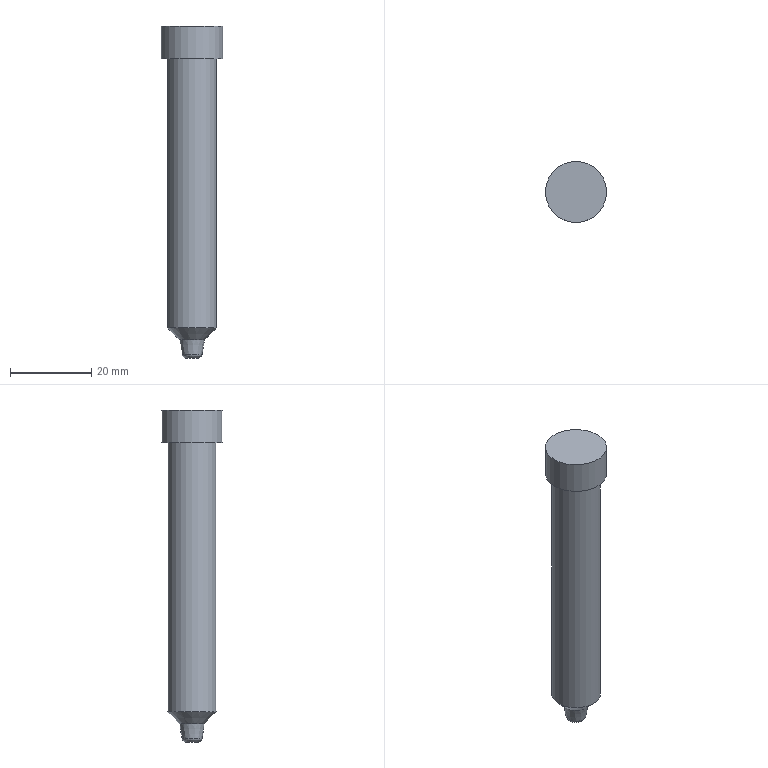Part | NX | features solid 2 | 1 solid | 8 faces | box 15 x 15 x 81.5 mm | volume 9187 mm3 | plane 3 | cylinder 2 | cone 2 | torus 1 | commonest cylinder face diameters 12 x1 15 x1
STEP:
#1=CARTESIAN_POINT('',(3119.266,-809.537,871.616));
#2=VERTEX_POINT('',#1);
#3=CARTESIAN_POINT('',(3113.266,-809.537,871.616));
#4=DIRECTION('',(0.,0.,1.));
#5=DIRECTION('',(1.,0.,0.));
#6=AXIS2_PLACEMENT_3D('',#3,#4,#5);
#7=CIRCLE('',#6,6.);
#8=EDGE_CURVE('',#2,#2,#7,.T.);
#9=ORIENTED_EDGE('',*,*,#8,.T.);
#10=EDGE_LOOP('',(#9));
#11=FACE_BOUND('',#10,.T.);
#12=CARTESIAN_POINT('',(3119.266,-809.537,937.716));
#13=VERTEX_POINT('',#12);
#14=CARTESIAN_POINT('',(3113.266,-809.537,937.716));
#15=DIRECTION('',(0.,0.,1.));
#16=DIRECTION('',(1.,0.,0.));
#17=AXIS2_PLACEMENT_3D('',#14,#15,#16);
#18=CIRCLE('',#17,6.);
#19=EDGE_CURVE('',#13,#13,#18,.F.);
#20=ORIENTED_EDGE('',*,*,#19,.T.);
#21=EDGE_LOOP('',(#20));
#22=FACE_BOUND('',#21,.T.);
#23=CARTESIAN_POINT('',(3113.266,-809.537,948.716));
#24=DIRECTION('',(0.,0.,-1.));
#25=DIRECTION('',(-1.,0.,0.));
#26=AXIS2_PLACEMENT_3D('',#23,#24,#25);
#27=CYLINDRICAL_SURFACE('',#26,6.);
#28=ADVANCED_FACE('',(#11,#22),#27,.T.);
#29=CARTESIAN_POINT('',(3116.369,-809.537,868.72));
#30=VERTEX_POINT('',#29);
#31=CARTESIAN_POINT('',(3113.266,-809.537,868.72));
#32=DIRECTION('',(0.,0.,1.));
#33=DIRECTION('',(1.,0.,0.));
#34=AXIS2_PLACEMENT_3D('',#31,#32,#33);
#35=CIRCLE('',#34,3.103);
#36=EDGE_CURVE('',#30,#30,#35,.F.);
#37=ORIENTED_EDGE('',*,*,#36,.T.);
#38=EDGE_LOOP('',(#37));
#39=FACE_BOUND('',#38,.T.);
#40=CARTESIAN_POINT('',(3113.266,-811.992,865.043));
#41=VERTEX_POINT('',#40);
#42=CARTESIAN_POINT('',(3113.266,-809.537,865.043));
#43=DIRECTION('',(0.,0.,1.));
#44=DIRECTION('',(0.,-1.,0.));
#45=AXIS2_PLACEMENT_3D('',#42,#43,#44);
#46=CIRCLE('',#45,2.455);
#47=EDGE_CURVE('',#41,#41,#46,.T.);
#48=ORIENTED_EDGE('',*,*,#47,.T.);
#49=EDGE_LOOP('',(#48));
#50=FACE_BOUND('',#49,.T.);
#51=CARTESIAN_POINT('',(3113.266,-809.537,866.237));
#52=DIRECTION('',(0.,0.,1.));
#53=DIRECTION('',(0.,1.,0.));
#54=AXIS2_PLACEMENT_3D('',#51,#52,#53);
#55=CONICAL_SURFACE('',#54,2.666,0.1745);
#56=ADVANCED_FACE('',(#39,#50),#55,.T.);
#57=CARTESIAN_POINT('',(3113.266,-811.037,864.217));
#58=VERTEX_POINT('',#57);
#59=CARTESIAN_POINT('',(3113.266,-809.537,864.217));
#60=DIRECTION('',(0.,0.,1.));
#61=DIRECTION('',(0.,-1.,0.));
#62=AXIS2_PLACEMENT_3D('',#59,#60,#61);
#63=CIRCLE('',#62,1.5);
#64=EDGE_CURVE('',#58,#58,#63,.T.);
#65=ORIENTED_EDGE('',*,*,#64,.T.);
#66=EDGE_LOOP('',(#65));
#67=FACE_BOUND('',#66,.T.);
#68=ORIENTED_EDGE('',*,*,#47,.F.);
#69=EDGE_LOOP('',(#68));
#70=FACE_BOUND('',#69,.T.);
#71=CARTESIAN_POINT('',(3113.266,-809.537,865.216));
#72=DIRECTION('',(0.,0.,-1.));
#73=DIRECTION('',(0.,-1.,0.));
#74=AXIS2_PLACEMENT_3D('',#71,#72,#73);
#75=TOROIDAL_SURFACE('',#74,1.47,1.);
#76=ADVANCED_FACE('',(#67,#70),#75,.T.);
#77=ORIENTED_EDGE('',*,*,#64,.F.);
#78=EDGE_LOOP('',(#77));
#79=FACE_BOUND('',#78,.T.);
#80=CARTESIAN_POINT('',(3113.266,-809.537,864.217));
#81=DIRECTION('',(0.,0.,-1.));
#82=DIRECTION('',(-1.,0.,0.));
#83=AXIS2_PLACEMENT_3D('',#80,#81,#82);
#84=PLANE('',#83);
#85=ADVANCED_FACE('',(#79),#84,.T.);
#86=CARTESIAN_POINT('',(3120.766,-809.537,945.716));
#87=VERTEX_POINT('',#86);
#88=CARTESIAN_POINT('',(3113.266,-809.537,945.716));
#89=DIRECTION('',(0.,0.,1.));
#90=DIRECTION('',(1.,0.,0.));
#91=AXIS2_PLACEMENT_3D('',#88,#89,#90);
#92=CIRCLE('',#91,7.5);
#93=EDGE_CURVE('',#87,#87,#92,.T.);
#94=ORIENTED_EDGE('',*,*,#93,.T.);
#95=EDGE_LOOP('',(#94));
#96=FACE_BOUND('',#95,.T.);
#97=CARTESIAN_POINT('',(2656.665,-762.453,945.716));
#98=DIRECTION('',(0.,0.,1.));
#99=DIRECTION('',(1.,0.,0.));
#100=AXIS2_PLACEMENT_3D('',#97,#98,#99);
#101=PLANE('',#100);
#102=ADVANCED_FACE('',(#96),#101,.T.);
#103=CARTESIAN_POINT('',(3120.766,-809.537,937.716));
#104=VERTEX_POINT('',#103);
#105=CARTESIAN_POINT('',(3113.266,-809.537,937.716));
#106=DIRECTION('',(0.,0.,1.));
#107=DIRECTION('',(1.,0.,0.));
#108=AXIS2_PLACEMENT_3D('',#105,#106,#107);
#109=CIRCLE('',#108,7.5);
#110=EDGE_CURVE('',#104,#104,#109,.T.);
#111=ORIENTED_EDGE('',*,*,#110,.T.);
#112=EDGE_LOOP('',(#111));
#113=FACE_BOUND('',#112,.T.);
#114=ORIENTED_EDGE('',*,*,#93,.F.);
#115=EDGE_LOOP('',(#114));
#116=FACE_BOUND('',#115,.T.);
#117=CARTESIAN_POINT('',(3113.266,-809.537,958.716));
#118=DIRECTION('',(0.,0.,-1.));
#119=DIRECTION('',(-1.,0.,0.));
#120=AXIS2_PLACEMENT_3D('',#117,#118,#119);
#121=CYLINDRICAL_SURFACE('',#120,7.5);
#122=ADVANCED_FACE('',(#113,#116),#121,.T.);
#123=ORIENTED_EDGE('',*,*,#19,.F.);
#124=EDGE_LOOP('',(#123));
#125=FACE_BOUND('',#124,.T.);
#126=ORIENTED_EDGE('',*,*,#110,.F.);
#127=EDGE_LOOP('',(#126));
#128=FACE_BOUND('',#127,.T.);
#129=CARTESIAN_POINT('',(3113.266,-809.537,937.716));
#130=DIRECTION('',(0.,0.,1.));
#131=DIRECTION('',(1.,0.,0.));
#132=AXIS2_PLACEMENT_3D('',#129,#130,#131);
#133=PLANE('',#132);
#134=ADVANCED_FACE('',(#125,#128),#133,.F.);
#135=ORIENTED_EDGE('',*,*,#36,.F.);
#136=EDGE_LOOP('',(#135));
#137=FACE_BOUND('',#136,.T.);
#138=ORIENTED_EDGE('',*,*,#8,.F.);
#139=EDGE_LOOP('',(#138));
#140=FACE_BOUND('',#139,.T.);
#141=CARTESIAN_POINT('',(3113.266,-809.537,871.616));
#142=DIRECTION('',(0.,0.,1.));
#143=DIRECTION('',(1.,0.,0.));
#144=AXIS2_PLACEMENT_3D('',#141,#142,#143);
#145=CONICAL_SURFACE('',#144,6.,0.7854);
#146=ADVANCED_FACE('',(#137,#140),#145,.T.);
#147=CLOSED_SHELL('',(#28,#56,#76,#85,#102,#122,#134,#146));
#148=MANIFOLD_SOLID_BREP('',#147);
#149=(LENGTH_UNIT()NAMED_UNIT(*)SI_UNIT(.MILLI.,.METRE.));
#150=UNCERTAINTY_MEASURE_WITH_UNIT(LENGTH_MEASURE(0.00001),#149,'','');
#151=(NAMED_UNIT(*)PLANE_ANGLE_UNIT()SI_UNIT($,.RADIAN.));
#152=(NAMED_UNIT(*)SI_UNIT($,.STERADIAN.)SOLID_ANGLE_UNIT());
#153=(GEOMETRIC_REPRESENTATION_CONTEXT(3)GLOBAL_UNCERTAINTY_ASSIGNED_CONTEXT((#150))GLOBAL_UNIT_ASSIGNED_CONTEXT((#149,#151,#152))REPRESENTATION_CONTEXT('',''));
#154=ADVANCED_BREP_SHAPE_REPRESENTATION('',(#148),#153);